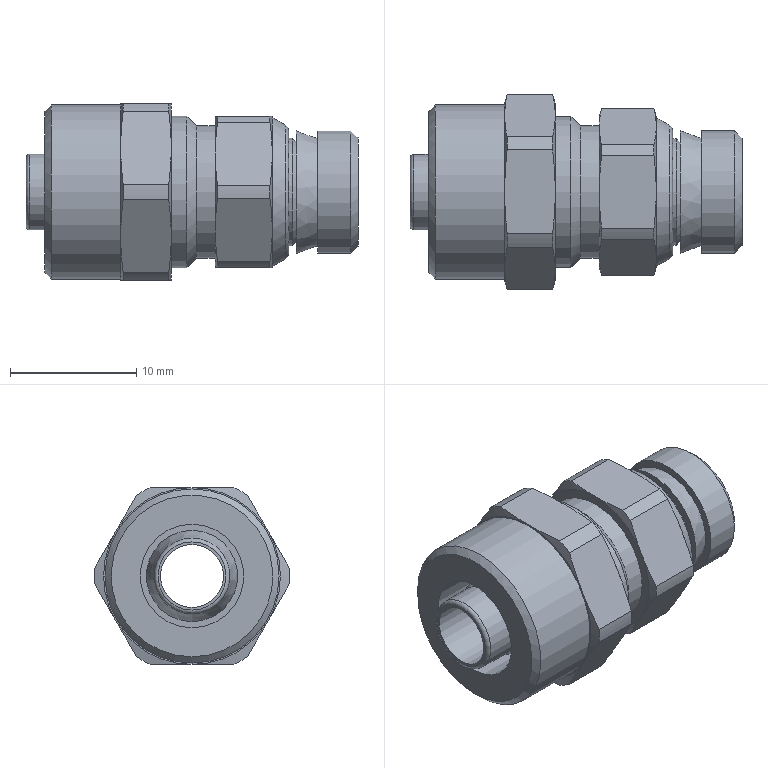Part | STEP file | Fitting | 1 solid | 77 faces | box 26.3 x 15.5 x 14 mm | volume 2394 mm3 | cone 31 | plane 23 | cylinder 21 | torus 2 | commonest cylinder face diameters 13.3 x6 15.5 x6 5 x1 6 x1 7.235 x1 8.2 x1